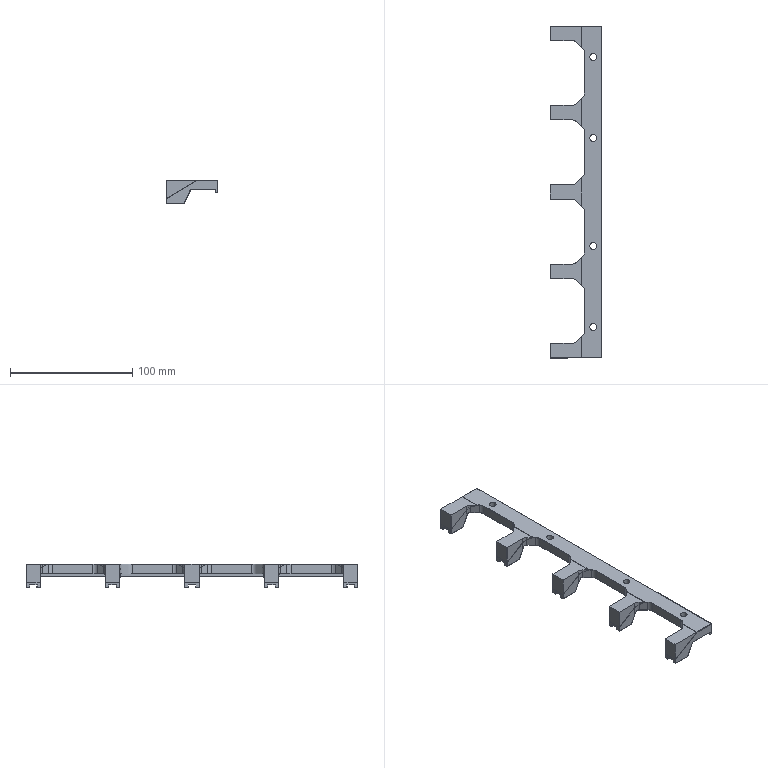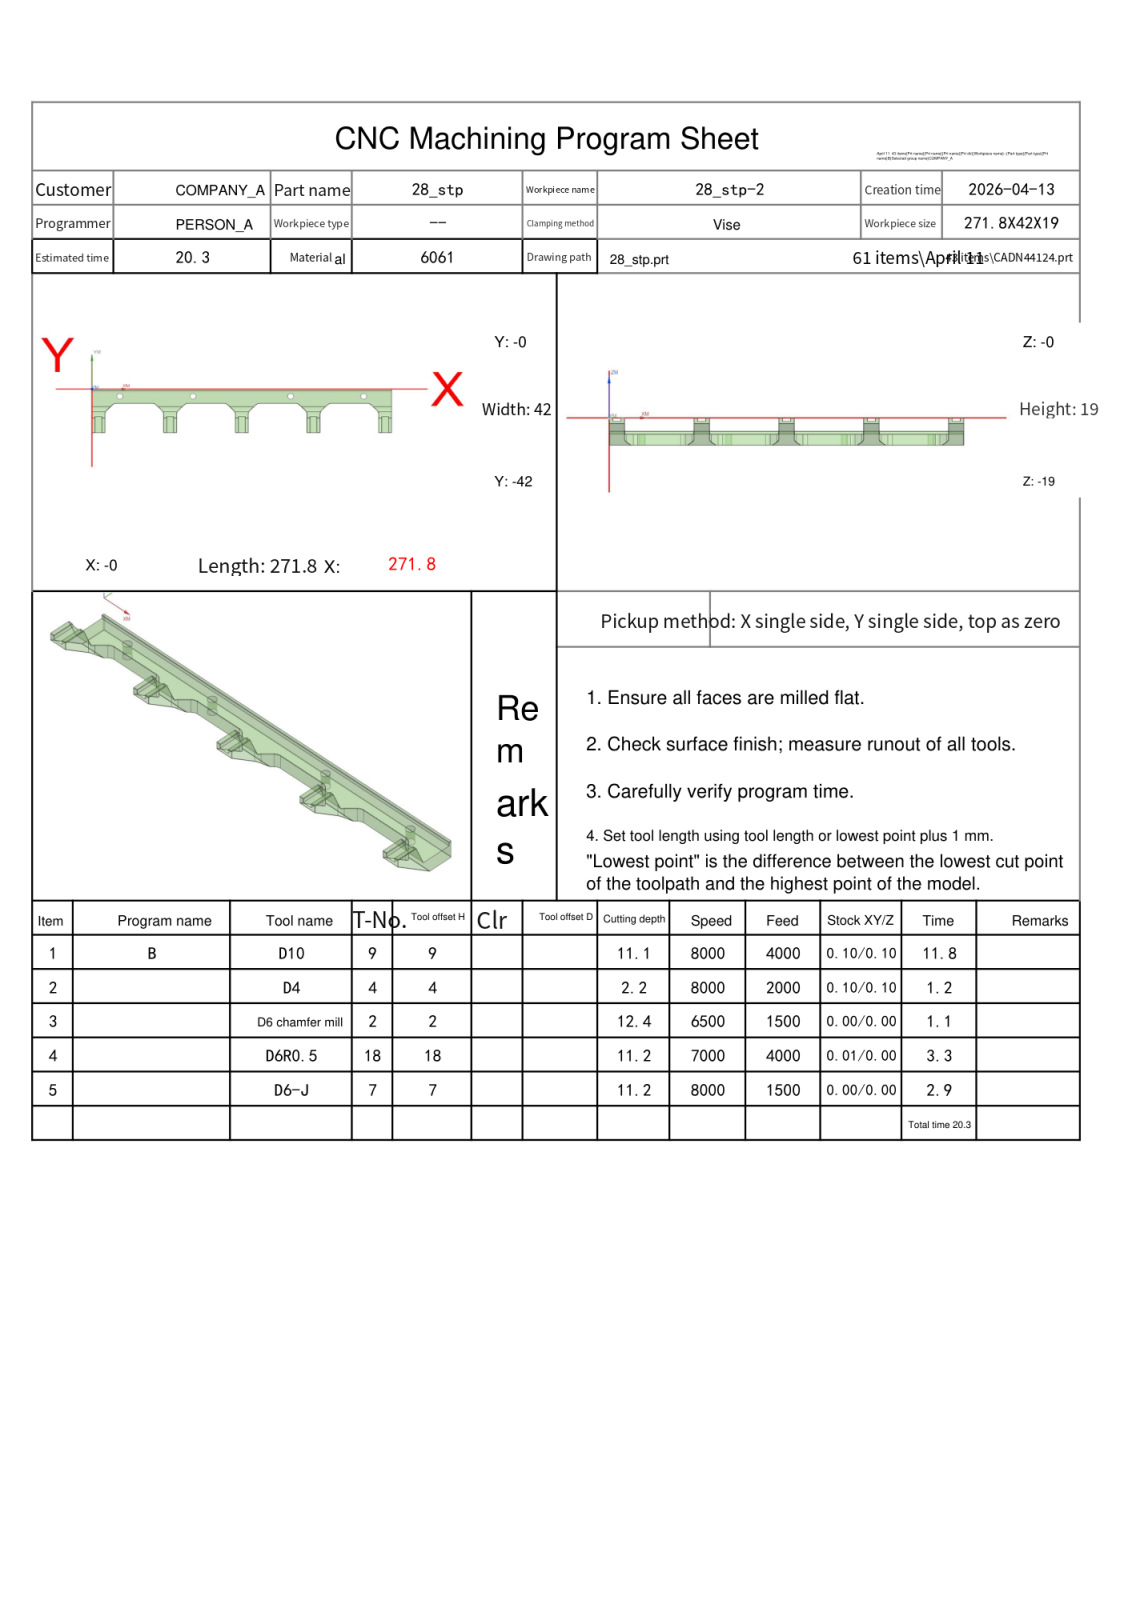NC program | NX | posted by the shop | part box 42 x 271.8 x 19 mm
Lines 7628 to 8696 of 14465:
N4 T18 M06
(D6R0.5  D=6. R=0.5 H=18 ce=0.01 di=0.00)
G00 G90 G54 X253.27 Y-27.629 M03 S7000
G43 H18 Z15.8
M08
Z.447
G01 Z-.053 F4000.
G03 X254.609 Y-27.944 I1.338 J2.685
X256.92 Y-26.857 I0.0 J3.
G02 X257.736 Y-25.975 I8.281 J-6.85
X259.802 Y-25.09 I2.255 J-2.408
G01 X262.9 Y-25.088
G02 X264.966 Y-25.891 I-.055 J-3.199
X265.858 Y-26.823 I-6.91 J-7.504
G01 X265.898 Y-26.869
X265.915 Y-26.85
G02 X266.687 Y-26.023 I12.598 J-10.979
X268.753 Y-25.092 I2.328 J-2.409
G01 X268.925 Y-25.088
X271.734
G02 X273.985 Y-25.998 I0.0 J-3.24
X274.759 Y-26.825 I-7.84 J-8.116
G01 Y-26.799 Z-.105
G03 X273.917 Y-25.896 I-10.451 J-8.901
X271.748 Y-25.003 I-2.234 J-2.346
G01 X268.952
G03 X266.725 Y-25.95 I.099 J-3.323
X265.898 Y-26.843 I15.388 J-15.091
G01 X265.858 Y-26.797
G03 X264.966 Y-25.852 I-9.175 J-7.76
X262.848 Y-25.003 I-2.177 J-2.366
G01 X259.952
G03 X257.736 Y-25.938 I.084 J-3.291
X256.92 Y-26.831 I8.923 J-8.978
G01 Y-26.805 Z-.158
G02 X257.736 Y-25.906 I11.122 J-9.282
X260.004 Y-24.918 I2.338 J-2.269
G01 X262.796
G02 X264.966 Y-25.812 I-.092 J-3.303
G01 X265.111 Y-25.95
X265.736 Y-26.634
X265.859 Y-26.772
X265.898 Y-26.816
X266.686 Y-25.95
G02 X269.004 Y-24.918 I2.434 J-2.345
G01 X271.696
G02 X273.917 Y-25.859 I-.094 J-3.315
G01 X274.012 Y-25.95
X274.762 Y-26.776
Y-26.75 Z-.21
X274.04 Y-25.95
X273.917 Y-25.822
G03 X271.643 Y-24.833 I-2.386 J-2.377
G01 X269.057
G03 X266.661 Y-25.95 I.089 J-3.316
G01 X265.898 Y-26.79
X265.859 Y-26.746
X265.144 Y-25.95
X264.966 Y-25.773
G03 X262.743 Y-24.833 I-2.303 J-2.346
G01 X260.057
G03 X258.021 Y-25.608 I.064 J-3.227
G01 X257.736 Y-25.874
X257.657 Y-25.95
X257.041 Y-26.634
X256.92 Y-26.779
X256.919 Y-26.752 Z-.264
G02 X257.974 Y-25.608 I12.038 J-10.043
X260.112 Y-24.747 I2.203 J-2.384
G01 X262.691
G02 X264.966 Y-25.738 I-.091 J-3.317
X265.86 Y-26.72 I-21.948 J-20.865
G01 X265.898 Y-26.763
X266.636 Y-25.95
X266.687 Y-25.887
X266.974 Y-25.608
G02 X269.104 Y-24.747 I2.207 J-2.395
G01 X271.594
G02 X273.917 Y-25.791 I-.094 J-3.315
G01 X274.068 Y-25.95
X274.763 Y-26.724
Y-26.692 Z-.328
X273.917 Y-25.753
X273.774 Y-25.608
G03 X271.598 Y-24.669 I-2.244 J-2.208
G01 X269.106
G03 X266.952 Y-25.585 I.064 J-3.141
X265.898 Y-26.731 I18.412 J-17.995
G01 X265.86 Y-26.688
X265.078 Y-25.822
G03 X264.276 Y-25.138 I-2.992 J-2.699
X262.697 Y-24.669 I-1.588 J-2.453
G01 X260.1
G03 X257.926 Y-25.608 I.079 J-3.17
G01 X257.736 Y-25.803
X256.988 Y-26.634
X256.918 Y-26.719
X256.917 Y-26.679 Z-.407
X256.953 Y-26.634
X257.676 Y-25.827
X257.762 Y-25.73
G02 X258.405 Y-25.15 I2.847 J-2.508
X260.104 Y-24.606 I1.699 J-2.381
G01 X262.689
X262.699
G02 X264.469 Y-25.203 I0.0 J-2.924
X264.957 Y-25.648 I-2.232 J-2.934
G01 X265.31 Y-26.034
X265.861 Y-26.65
X265.898 Y-26.692
X265.953 Y-26.634
X266.676 Y-25.827
X266.762 Y-25.73
G02 X267.261 Y-25.257 I3.183 J-2.858
X269.107 Y-24.606 I1.852 J-2.308
G01 X271.592
G02 X273.824 Y-25.608 I-.022 J-3.035
G01 X273.917 Y-25.708
X274.764 Y-26.654
X274.696 Y-26.533 Z-.495
X274.024 Y-25.782
X273.85 Y-25.587
G03 X271.6 Y-24.558 I-2.275 J-2.001
G01 X269.093
G03 X266.982 Y-25.452 I0.0 J-2.941
G01 X266.85 Y-25.587
X266.676 Y-25.782
X265.956 Y-26.587
X265.898 Y-26.648
X265.77 Y-26.505
X264.977 Y-25.618
X264.95 Y-25.587
G03 X262.7 Y-24.558 I-2.275 J-2.001
G01 X260.1
G03 X257.85 Y-25.587 I.026 J-3.03
G01 X257.676 Y-25.782
X256.914 Y-26.634
X256.916 Y-26.591 Z-.585
X257.048 Y-26.44
X257.676 Y-25.738
X257.868 Y-25.523
G02 X260.1 Y-24.514 I2.244 J-1.991
G01 X262.7
G02 X264.932 Y-25.523 I-.012 J-3.
G01 X265.016 Y-25.617
X265.776 Y-26.467
X265.898 Y-26.603
X265.999 Y-26.494
X266.676 Y-25.738
X266.876 Y-25.514
G02 X267.029 Y-25.359 I4.931 J-4.721
X269.099 Y-24.514 I2.07 J-2.112
G01 X271.6
G02 X273.832 Y-25.523 I-.012 J-3.
G01 X274.024 Y-25.738
X274.605 Y-26.387
X274.714 Y-26.511
X274.725 Y-26.498 Z-.629
X274.733 Y-26.488 Z-.674
X274.605 Y-26.342
X274.024 Y-25.693
X273.826 Y-25.471
G03 X271.6 Y-24.469 I-2.234 J-1.988
G01 X269.097
G03 X267.121 Y-25.228 I0.0 J-2.95
X266.876 Y-25.469 I2.648 J-2.937
G01 X266.676 Y-25.693
X265.999 Y-26.45
X265.898 Y-26.558
X265.779 Y-26.425
X265.049 Y-25.608
X264.926 Y-25.472
G03 X262.7 Y-24.469 I-2.234 J-1.988
G01 X260.1
G03 X257.874 Y-25.472 I.008 J-2.99
G01 X257.676 Y-25.693
X257.048 Y-26.395
X256.917 Y-26.548
Y-26.504 Z-.763
X257.048 Y-26.35
X257.676 Y-25.648
X257.876 Y-25.425
G02 X260.1 Y-24.424 I2.231 J-1.987
G01 X262.7
G02 X264.924 Y-25.425 I-.006 J-2.987
G01 X265.089 Y-25.608
X265.799 Y-26.403
X265.898 Y-26.513
X265.999 Y-26.405
X266.676 Y-25.648
X266.876 Y-25.425
G02 X269.1 Y-24.424 I2.252 J-2.035
G01 X271.6
G02 X273.824 Y-25.425 I-.006 J-2.987
G01 X274.024 Y-25.648
X274.751 Y-26.466
X274.786 Y-26.463 Z-.853
X274.641 Y-26.292
X274.024 Y-25.604
X273.824 Y-25.38
G03 X271.6 Y-24.38 I-2.231 J-1.987
G01 X269.1
G03 X266.876 Y-25.38 I.006 J-2.987
G01 X266.676 Y-25.604
X265.999 Y-26.36
X265.898 Y-26.469
X265.819 Y-26.38
X265.124 Y-25.604
X264.924 Y-25.38
G03 X262.7 Y-24.38 I-2.231 J-1.987
G01 X260.1
G03 X257.876 Y-25.38 I.006 J-2.987
G01 X257.676 Y-25.604
X257.048 Y-26.306
X256.917 Y-26.46
Y-26.416 Z-.942
X257.02 Y-26.292
X257.676 Y-25.559
X257.876 Y-25.335
G02 X260.1 Y-24.335 I2.231 J-1.987
G01 X262.7
G02 X264.924 Y-25.335 I-.006 J-2.987
G01 X265.124 Y-25.559
X265.839 Y-26.358
X265.898 Y-26.424
X265.999 Y-26.316
X266.676 Y-25.559
X266.876 Y-25.335
G02 X269.1 Y-24.335 I2.231 J-1.987
G01 X271.6
G02 X273.824 Y-25.335 I-.006 J-2.987
G01 X274.024 Y-25.559
X274.681 Y-26.292
X274.815 Y-26.453
X274.829 Y-26.438 Z-.987
X274.835 Y-26.43 Z-1.032
X274.721 Y-26.292
X274.024 Y-25.514
X273.824 Y-25.29
G03 X271.6 Y-24.29 I-2.231 J-1.987
G01 X269.1
G03 X266.876 Y-25.29 I.006 J-2.987
G01 X266.676 Y-25.514
X265.98 Y-26.292
X265.898 Y-26.379
X265.859 Y-26.336
X265.124 Y-25.514
X264.924 Y-25.29
G03 X262.7 Y-24.29 I-2.231 J-1.987
G01 X260.1
G03 X257.876 Y-25.29 I.006 J-2.987
G01 X257.676 Y-25.514
X256.98 Y-26.292
X256.915 Y-26.371
X256.913 Y-26.325 Z-1.121
X256.939 Y-26.292
X257.676 Y-25.469
X257.876 Y-25.246
G02 X260.1 Y-24.245 I2.231 J-1.987
G01 X262.7
G02 X264.924 Y-25.246 I-.006 J-2.987
G01 X265.124 Y-25.469
X265.88 Y-26.313
X265.884 Y-26.34
X265.914
X265.919 Y-26.313
X265.939 Y-26.292
X266.676 Y-25.469
X266.876 Y-25.246
G02 X269.1 Y-24.245 I2.231 J-1.987
G01 X271.6
G02 X273.824 Y-25.246 I-.006 J-2.987
G01 X274.024 Y-25.469
X274.761 Y-26.292
X274.855 Y-26.408
X274.77 Y-26.26 Z-1.211
X274.024 Y-25.425
X273.824 Y-25.201
G03 X271.6 Y-24.201 I-2.231 J-1.987
G01 X269.1
G03 X266.865 Y-25.213 I.014 J-3.005
G01 X266.676 Y-25.425
X265.94 Y-26.247
X265.9 Y-26.292
X265.779 Y-26.157
X265.124 Y-25.425
X264.924 Y-25.201
G03 X262.7 Y-24.201 I-2.231 J-1.987
G01 X260.1
G03 X257.876 Y-25.201 I.006 J-2.987
G01 X257.676 Y-25.425
X256.912 Y-26.28
X256.913 Y-26.237 Z-1.3
X257.048 Y-26.082
X257.676 Y-25.38
X257.876 Y-25.156
G02 X260.1 Y-24.156 I2.231 J-1.987
G01 X262.7
G02 X264.924 Y-25.156 I-.006 J-2.987
G01 X265.124 Y-25.38
X265.673 Y-25.993
X265.9 Y-26.247
X265.99 Y-26.147
X266.676 Y-25.38
X266.818 Y-25.22
X266.792 Y-25.191
X266.822 Y-25.158
X266.854 Y-25.181
X266.876 Y-25.156
G02 X269.1 Y-24.156 I2.231 J-1.987
G01 X271.6
G02 X273.824 Y-25.156 I-.006 J-2.987
G01 X274.024 Y-25.38
X274.769 Y-26.217
Y-26.174 Z-1.39
X274.024 Y-25.335
X273.824 Y-25.112
G03 X271.6 Y-24.111 I-2.231 J-1.987
G01 X269.1
G03 X268.395 Y-24.194 I.011 J-3.136
G01 X268.534 Y-24.157 Z-1.407
X268.674 Y-24.124 Z-1.425
X268.816 Y-24.098 Z-1.443
X268.958 Y-24.079 Z-1.461
X269.1 Y-24.066 Z-1.479
X271.6
G02 X273.824 Y-25.067 I-.012 J-3.
G01 X274.024 Y-25.291
X274.769 Y-26.131
X274.77 Y-26.087 Z-1.568
X274.655 Y-25.95
X274.024 Y-25.246
X273.824 Y-25.022
G03 X271.6 Y-24.022 I-2.233 J-1.992
G01 X269.1
G00 Z15.8
X253.277 Y-26.914
Z-.89
G01 Z-1.39
G03 X254.637 Y-27.24 I1.359 J2.674
X256.914 Y-26.193 I0.0 J3.
G01 X257.048 Y-26.037
X257.676 Y-25.335
X257.876 Y-25.112
G02 X260.1 Y-24.111 I2.231 J-1.987
G01 X262.7
G02 X263.406 Y-24.194 I-.092 J-3.829
G01 X263.267 Y-24.157 Z-1.407
X263.126 Y-24.124 Z-1.425
X262.984 Y-24.098 Z-1.443
X262.842 Y-24.079 Z-1.461
X262.7 Y-24.066 Z-1.479
X260.1
G03 X257.876 Y-25.067 I.006 J-2.987
G01 X257.676 Y-25.291
X257.048 Y-25.992
X256.914 Y-26.15
Y-26.106 Z-1.568
X257.045 Y-25.95
X257.676 Y-25.246
X257.876 Y-25.022
G02 X260.1 Y-24.022 I2.231 J-1.987
G01 X262.7
G00 Z15.8
X278.416 Y-26.795
Z-1.158
G01 Z-1.658
G02 X277.07 Y-27.114 I-1.346 J2.681
X274.772 Y-26.042 I0.0 J3.
G01 X274.695 Y-25.95
X274.024 Y-25.201
X273.824 Y-24.977
G03 X271.6 Y-23.977 I-2.231 J-1.987
G01 X260.1
G03 X257.876 Y-24.977 I.006 J-2.987
G01 X257.676 Y-25.201
X257.005 Y-25.95
X256.913 Y-26.061
X256.912 Y-26.016 Z-1.747
X256.965 Y-25.95
X257.676 Y-25.156
X257.876 Y-24.933
G02 X260.1 Y-23.932 I2.231 J-1.987
G01 X271.6
G02 X273.824 Y-24.933 I-.006 J-2.987
G01 X274.024 Y-25.156
X274.735 Y-25.95
X274.774 Y-25.997
X274.776 Y-25.952 Z-1.837
X274.024 Y-25.112
X273.824 Y-24.888
G03 X271.6 Y-23.888 I-2.231 J-1.987
G01 X260.1
G03 X257.876 Y-24.888 I.006 J-2.987
G01 X257.676 Y-25.112
X256.925 Y-25.95
X256.91 Y-25.97
X256.909 Y-25.926 Z-1.926
X257.048 Y-25.769
X257.676 Y-25.067
X257.876 Y-24.843
G02 X260.1 Y-23.843 I2.231 J-1.987
G01 X271.6
G02 X273.824 Y-24.843 I-.006 J-2.987
G01 X274.024 Y-25.067
X274.775 Y-25.909
Y-25.866 Z-2.016
X274.024 Y-25.022
X273.824 Y-24.799
G03 X271.6 Y-23.798 I-2.231 J-1.987
G01 X260.1
G03 X257.876 Y-24.799 I.006 J-2.987
G01 X257.676 Y-25.022
X257.048 Y-25.724
X256.911 Y-25.882
Y-25.839 Z-2.105
X257.048 Y-25.679
X257.676 Y-24.977
X257.876 Y-24.754
G02 X260.1 Y-23.753 I2.231 J-1.987
G01 X271.6
G02 X273.824 Y-24.754 I-.006 J-2.987
G01 X274.024 Y-24.977
X274.775 Y-25.823
Y-25.779 Z-2.195
X274.629 Y-25.608
X274.024 Y-24.933
X273.824 Y-24.709
G03 X271.6 Y-23.709 I-2.238 J-2.003
G01 X260.1
G03 X257.876 Y-24.709 I.006 J-2.987
G01 X257.676 Y-24.933
X257.048 Y-25.635
X256.912 Y-25.795
Y-25.751 Z-2.284
X257.031 Y-25.608
X257.876 Y-24.664
G02 X260.1 Y-23.664 I2.231 J-1.987
G01 X271.6
G02 X273.824 Y-24.664 I-.006 J-2.987
G01 X274.024 Y-24.888
X274.669 Y-25.608
X274.776 Y-25.735
X274.778 Y-25.69 Z-2.373
X274.709 Y-25.608
X274.024 Y-24.843
X273.824 Y-24.62
G03 X271.6 Y-23.619 I-2.231 J-1.987
G01 X260.1
G03 X257.876 Y-24.62 I.006 J-2.987
G01 X256.991 Y-25.608
X256.911 Y-25.706
X256.909 Y-25.66 Z-2.463
X256.951 Y-25.608
X257.876 Y-24.575
G02 X260.1 Y-23.575 I2.231 J-1.987
G01 X271.6
G02 X273.824 Y-24.575 I-.006 J-2.987
G01 X274.024 Y-24.799
X274.749 Y-25.608
X274.78 Y-25.645
X274.782 Y-25.6 Z-2.552
X274.024 Y-24.754
X273.824 Y-24.53
G03 X271.6 Y-23.53 I-2.231 J-1.987
G01 X260.1
G03 X257.876 Y-24.53 I.006 J-2.987
G01 X257.676 Y-24.754
X256.907 Y-25.614
X256.908 Y-25.571 Z-2.642
X257.048 Y-25.411
X257.876 Y-24.485
G02 X260.1 Y-23.485 I2.231 J-1.987
G01 X271.6
G02 X273.824 Y-24.485 I-.006 J-2.987
G01 X274.024 Y-24.709
X274.781 Y-25.558
X274.78 Y-25.514 Z-2.731
X274.024 Y-24.664
X273.824 Y-24.441
G03 X271.6 Y-23.44 I-2.231 J-1.987
G01 X260.1
G03 X257.876 Y-24.441 I.006 J-2.987
G01 X257.048 Y-25.366
X256.909 Y-25.528
Y-25.484 Z-2.821
X257.048 Y-25.322
X257.876 Y-24.396
G02 X260.1 Y-23.396 I2.231 J-1.987
G01 X271.6
G02 X273.824 Y-24.396 I-.009 J-2.992
G01 X274.024 Y-24.62
X274.78 Y-25.471
X274.781 Y-25.427 Z-2.91
X274.643 Y-25.266
X274.024 Y-24.575
X273.824 Y-24.351
G03 X271.6 Y-23.351 I-2.237 J-2.001
G01 X260.1
G03 X257.876 Y-24.351 I.006 J-2.987
G01 X257.048 Y-25.277
X256.91 Y-25.44
X256.909 Y-25.395 Z-3.
X257.017 Y-25.266
X257.876 Y-24.307
G02 X260.1 Y-23.306 I2.231 J-1.987
G01 X271.6
G02 X273.824 Y-24.307 I-.006 J-2.987
G01 X274.024 Y-24.53
X274.683 Y-25.266
X274.782 Y-25.382
X274.783 Y-25.338 Z-3.089
X274.723 Y-25.266
X274.024 Y-24.486
X273.824 Y-24.262
G03 X271.6 Y-23.261 I-2.231 J-1.987
G01 X260.1
G03 X257.876 Y-24.262 I.006 J-2.987
G01 X256.977 Y-25.266
X256.908 Y-25.35
X256.906 Y-25.304 Z-3.178
X256.937 Y-25.266
X257.876 Y-24.217
G02 X260.1 Y-23.217 I2.231 J-1.987
G01 X271.6
G02 X273.824 Y-24.217 I-.006 J-2.987
G01 X274.024 Y-24.441
X274.763 Y-25.266
X274.785 Y-25.292
X274.786 Y-25.248 Z-3.268
X274.024 Y-24.396
X273.824 Y-24.172
G03 X271.6 Y-23.172 I-2.231 J-1.987
G01 X260.1
G03 X257.876 Y-24.172 I.006 J-2.987
G01 X257.676 Y-24.396
X256.904 Y-25.259
X256.906 Y-25.216 Z-3.357
X257.048 Y-25.053
X257.876 Y-24.128
G02 X260.1 Y-23.127 I2.231 J-1.987
G01 X271.6
G02 X273.824 Y-24.128 I-.006 J-2.987
G01 X274.024 Y-24.351
X274.785 Y-25.205
Y-25.162 Z-3.447
X274.024 Y-24.307
X273.824 Y-24.083
G03 X271.6 Y-23.083 I-2.231 J-1.987
G01 X260.1
G03 X257.876 Y-24.083 I.006 J-2.987
G01 X257.048 Y-25.009
X256.907 Y-25.172
Y-25.129 Z-3.536
X257.048 Y-24.964
X257.876 Y-24.038
G02 X260.1 Y-23.038 I2.231 J-1.987
G01 X271.6
G02 X273.824 Y-24.038 I-.012 J-3.001
G01 X274.024 Y-24.262
X274.785 Y-25.118
Y-25.074 Z-3.626
X274.657 Y-24.924
X274.024 Y-24.217
X273.824 Y-23.994
G03 X271.6 Y-22.993 I-2.232 J-1.989
G01 X260.1
G03 X257.876 Y-23.994 I.006 J-2.987
G01 X257.043 Y-24.924
X256.908 Y-25.085
X256.907 Y-25.04 Z-3.715
X257.003 Y-24.924
X257.876 Y-23.949
G02 X260.1 Y-22.948 I2.231 J-1.987
G01 X271.6
G02 X273.824 Y-23.949 I-.006 J-2.987
G01 X274.024 Y-24.172
X274.697 Y-24.924
X274.787 Y-25.03
X274.788 Y-24.985 Z-3.805
X274.738 Y-24.924
X274.024 Y-24.128
X273.824 Y-23.904
G03 X271.6 Y-22.904 I-2.231 J-1.987
G01 X260.1
G03 X257.876 Y-23.904 I.006 J-2.987
G01 X256.963 Y-24.924
X256.905 Y-24.994
X256.903 Y-24.949 Z-3.894
X256.923 Y-24.924
X257.876 Y-23.859
G02 X260.1 Y-22.859 I2.231 J-1.987
G01 X271.6
G02 X273.824 Y-23.859 I-.006 J-2.987
G01 X274.024 Y-24.083
X274.79 Y-24.94
Y-24.896 Z-3.983
X274.024 Y-24.038
X273.824 Y-23.815
G03 X271.6 Y-22.814 I-2.231 J-1.987
G01 X260.1
G03 X257.876 Y-23.815 I.006 J-2.987
G01 X257.048 Y-24.74
X256.903 Y-24.904
X256.904 Y-24.861 Z-4.073
X257.048 Y-24.695
X257.876 Y-23.77
G02 X260.1 Y-22.77 I2.231 J-1.987
G01 X271.6
G02 X273.824 Y-23.77 I-.006 J-2.987
G01 X274.024 Y-23.994
X274.789 Y-24.852
Y-24.809 Z-4.162
X274.024 Y-23.949
X273.824 Y-23.725
G03 X271.6 Y-22.725 I-2.231 J-1.987
G01 X260.1
G03 X257.876 Y-23.725 I.006 J-2.987
G01 X257.048 Y-24.651
X256.905 Y-24.817
X256.906 Y-24.773 Z-4.252
X257.048 Y-24.606
X257.876 Y-23.681
G02 X260.1 Y-22.68 I2.231 J-1.987
G01 X271.6
G02 X273.824 Y-23.681 I-.014 J-3.004
G01 X274.024 Y-23.904
X274.789 Y-24.765
Y-24.72 Z-4.341
X274.672 Y-24.582
X274.024 Y-23.859
X273.824 Y-23.636
G03 X271.6 Y-22.635 I-2.231 J-1.987
G01 X260.1
G03 X257.876 Y-23.636 I.006 J-2.987
G01 X257.029 Y-24.582
X256.906 Y-24.728
X256.905 Y-24.683 Z-4.431
X256.989 Y-24.582
X257.876 Y-23.591
G02 X260.1 Y-22.591 I2.231 J-1.987
G01 X271.6
G02 X273.824 Y-23.591 I-.006 J-2.987
G01 X274.024 Y-23.815
X274.712 Y-24.582
X274.79 Y-24.675
X274.792 Y-24.63 Z-4.52
X274.752 Y-24.582
X274.024 Y-23.77
X273.824 Y-23.546
G03 X271.6 Y-22.546 I-2.231 J-1.987
G01 X260.1
G03 X257.876 Y-23.546 I.006 J-2.987
G01 X256.949 Y-24.582
X256.904 Y-24.637
X256.902 Y-24.591 Z-4.609
X257.676 Y-23.725
X257.876 Y-23.502
G02 X260.1 Y-22.501 I2.231 J-1.987
G01 X271.6
G02 X273.824 Y-23.502 I-.006 J-2.987
G01 X274.024 Y-23.725
X274.793 Y-24.584
X274.792 Y-24.541 Z-4.699
X274.024 Y-23.681
X273.824 Y-23.457
G03 X271.6 Y-22.457 I-2.231 J-1.987
G01 X260.1
G03 X257.876 Y-23.457 I.006 J-2.987
G01 X257.048 Y-24.382
X256.903 Y-24.548
X256.904 Y-24.504 Z-4.788
X257.048 Y-24.338
X257.876 Y-23.412
G02 X260.1 Y-22.412 I2.231 J-1.987
G01 X271.6
G02 X273.824 Y-23.412 I-.006 J-2.987
G01 X274.024 Y-23.636
X274.792 Y-24.498
X274.791 Y-24.454 Z-4.878
X274.024 Y-23.591
X273.824 Y-23.367
G03 X271.6 Y-22.367 I-2.234 J-1.994
G01 X260.1
G03 X257.876 Y-23.367 I.006 J-2.987
G01 X257.048 Y-24.293
X256.905 Y-24.46
Y-24.416 Z-4.967
X257.048 Y-24.248
X257.876 Y-23.323
G02 X260.1 Y-22.322 I2.231 J-1.987
G01 X271.6
G02 X273.824 Y-23.323 I-.012 J-3.
G01 X274.024 Y-23.546
X274.646 Y-24.24
X274.791 Y-24.41
X274.792 Y-24.365 Z-5.057
X274.686 Y-24.24
X274.024 Y-23.502
X273.824 Y-23.278
G03 X271.6 Y-22.278 I-2.231 J-1.987
G01 X260.1
G03 X257.876 Y-23.278 I.006 J-2.987
G01 X257.015 Y-24.24
X256.905 Y-24.371
X256.904 Y-24.326 Z-5.146
X256.975 Y-24.24
X257.876 Y-23.233
G02 X260.1 Y-22.233 I2.231 J-1.987
G01 X271.6
G02 X273.824 Y-23.233 I-.006 J-2.987
G01 X274.024 Y-23.457
X274.726 Y-24.24
X274.793 Y-24.32
X274.795 Y-24.275 Z-5.236
X274.766 Y-24.24
X274.024 Y-23.412
X273.824 Y-23.189
G03 X271.6 Y-22.188 I-2.231 J-1.987
G01 X260.1
G03 X257.876 Y-23.189 I.006 J-2.987
G01 X256.935 Y-24.24
X256.902 Y-24.28
X256.901 Y-24.234 Z-5.325
X257.676 Y-23.367
X257.876 Y-23.144
G02 X260.1 Y-22.143 I2.231 J-1.987
G01 X271.6
G02 X273.824 Y-23.144 I-.006 J-2.987
G01 X274.024 Y-23.367
X274.796 Y-24.23
X274.794 Y-24.186 Z-5.414
X274.024 Y-23.323
X273.824 Y-23.099
G03 X271.6 Y-22.099 I-2.231 J-1.987
G01 X260.1
G03 X257.876 Y-23.099 I.006 J-2.987
G01 X257.048 Y-24.025
X256.902 Y-24.191
X256.903 Y-24.147 Z-5.504
X257.048 Y-23.98
X257.876 Y-23.054
G02 X260.1 Y-22.054 I2.231 J-1.987
G01 X271.6
G02 X273.824 Y-23.054 I-.006 J-2.987
G01 X274.024 Y-23.278
X274.794 Y-24.143
X274.793 Y-24.099 Z-5.593
X274.024 Y-23.233
X273.824 Y-23.01
G03 X271.6 Y-22.009 I-2.237 J-2.001
G01 X260.1
G03 X257.876 Y-23.01 I.006 J-2.987
G01 X257.048 Y-23.935
X256.904 Y-24.103
X256.905 Y-24.059 Z-5.683
X257.041 Y-23.898
X257.876 Y-22.965
G02 X260.1 Y-21.965 I2.231 J-1.987
G01 X271.6
G02 X273.824 Y-22.965 I-.006 J-2.987
G01 X274.024 Y-23.189
X274.66 Y-23.898
X274.793 Y-24.054
X274.794 Y-24.009 Z-5.772
X274.7 Y-23.898
X274.024 Y-23.144
X273.824 Y-22.92
G03 X271.6 Y-21.92 I-2.231 J-1.987
G01 X260.1
G03 X257.876 Y-22.92 I.006 J-2.987
G01 X257.001 Y-23.898
X256.904 Y-24.014
X256.903 Y-23.968 Z-5.862
X256.961 Y-23.898
X257.876 Y-22.876
G02 X260.1 Y-21.875 I2.231 J-1.987
G01 X271.6
G02 X273.824 Y-22.876 I-.006 J-2.987
G01 X274.024 Y-23.099
X274.74 Y-23.898
X274.795 Y-23.964
X274.796 Y-23.918 Z-5.951
X274.024 Y-23.054
X273.824 Y-22.831
G03 X271.6 Y-21.83 I-2.231 J-1.987
G01 X260.1
G03 X257.876 Y-22.831 I.006 J-2.987
G01 X256.921 Y-23.898
X256.901 Y-23.922
Y-23.877 Z-6.041
X257.048 Y-23.712
X257.876 Y-22.786
G02 X260.1 Y-21.786 I2.231 J-1.987
G01 X271.6
G02 X273.824 Y-22.786 I-.006 J-2.987
G01 X274.024 Y-23.01
X274.796 Y-23.874
X274.795 Y-23.83 Z-6.13
X274.024 Y-22.965
X273.824 Y-22.741
G03 X271.6 Y-21.741 I-2.231 J-1.987
G01 X260.1
G03 X257.876 Y-22.741 I.006 J-2.987
G01 X257.048 Y-23.667
X256.903 Y-23.834
X256.904 Y-23.79 Z-6.219
X257.048 Y-23.622
X257.876 Y-22.697
G02 X260.1 Y-21.696 I2.231 J-1.987
G01 X271.6
G02 X273.824 Y-22.697 I-.006 J-2.987
G01 X274.024 Y-22.92
X274.795 Y-23.786
X274.794 Y-23.742 Z-6.309
X274.024 Y-22.876
X273.824 Y-22.652
G03 X271.6 Y-21.652 I-2.238 J-2.003
G01 X260.1
G03 X257.876 Y-22.652 I.006 J-2.987
G01 X257.048 Y-23.577
X256.904 Y-23.746
X256.905 Y-23.701 Z-6.398
X257.027 Y-23.556
X257.876 Y-22.607
G02 X260.1 Y-21.607 I2.231 J-1.987
G01 X271.6
G02 X273.824 Y-22.607 I-.006 J-2.987
G01 X274.024 Y-22.831
X274.674 Y-23.556
X274.795 Y-23.697
Y-23.652 Z-6.488
X274.714 Y-23.556
X274.024 Y-22.786
X273.824 Y-22.562
G03 X271.6 Y-21.562 I-2.231 J-1.987
G01 X260.1
G03 X257.876 Y-22.562 I.006 J-2.987
G01 X256.987 Y-23.556
X256.904 Y-23.656
X256.903 Y-23.61 Z-6.577
X256.947 Y-23.556
X257.876 Y-22.518
G02 X260.1 Y-21.517 I2.231 J-1.987
G01 X271.6
G02 X273.824 Y-22.518 I-.006 J-2.987
G01 X274.024 Y-22.741
X274.754 Y-23.556
X274.796 Y-23.607
X274.798 Y-23.561 Z-6.667
X274.024 Y-22.697
X273.824 Y-22.473
G03 X271.6 Y-21.473 I-2.231 J-1.987
G01 X260.1
G03 X257.876 Y-22.473 I.006 J-2.987
G01 X257.676 Y-22.697
X256.901 Y-23.564
X256.902 Y-23.52 Z-6.756
X257.048 Y-23.354
X257.876 Y-22.428
G02 X260.1 Y-21.428 I2.231 J-1.987
G01 X271.6
G02 X273.824 Y-22.428 I-.006 J-2.987
G01 X274.024 Y-22.652
X274.797 Y-23.517
X274.796 Y-23.473 Z-6.846
X274.024 Y-22.607
X273.824 Y-22.384
G03 X271.6 Y-21.383 I-2.231 J-1.987
G01 X260.1
G03 X257.876 Y-22.384 I.006 J-2.987
G01 X257.048 Y-23.309
X256.903 Y-23.476
X256.904 Y-23.432 Z-6.935
X257.048 Y-23.264
X257.876 Y-22.339
G02 X260.1 Y-21.338 I2.231 J-1.987
G01 X271.6
G02 X273.824 Y-22.339 I-.01 J-2.995
G01 X274.024 Y-22.563
X274.795 Y-23.429
Y-23.385 Z-7.024
X274.648 Y-23.214
X274.024 Y-22.518
X273.824 Y-22.294
G03 X271.6 Y-21.294 I-2.236 J-1.998
G01 X260.1
G03 X257.876 Y-22.294 I.006 J-2.987
G01 X257.048 Y-23.22
X256.905 Y-23.388
Y-23.343 Z-7.114
X257.013 Y-23.214
X257.876 Y-22.249
G02 X260.1 Y-21.249 I2.231 J-1.987
G01 X271.6
G02 X273.824 Y-22.249 I-.006 J-2.987
G01 X274.024 Y-22.473
X274.688 Y-23.214
X274.795 Y-23.34
X274.796 Y-23.294 Z-7.203
X274.728 Y-23.214
X274.024 Y-22.428
X273.824 Y-22.205
G03 X271.6 Y-21.204 I-2.231 J-1.987
G01 X260.1
G03 X257.876 Y-22.205 I.006 J-2.987
G01 X256.973 Y-23.214
X256.904 Y-23.297
X256.903 Y-23.251 Z-7.293
X256.933 Y-23.214
X257.876 Y-22.16
G02 X260.1 Y-21.16 I2.231 J-1.987
G01 X271.6
G02 X273.824 Y-22.16 I-.006 J-2.987
G01 X274.024 Y-22.384
X274.768 Y-23.214
X274.797 Y-23.249
X274.798 Y-23.203 Z-7.382
X274.024 Y-22.339
X273.824 Y-22.115
G03 X271.6 Y-21.115 I-2.231 J-1.987
G01 X260.1
G03 X257.876 Y-22.115 I.006 J-2.987
G01 X257.676 Y-22.339
X256.901 Y-23.205
X256.903 Y-23.162 Z-7.472
X257.048 Y-22.996
X257.876 Y-22.071
G02 X260.1 Y-21.07 I2.231 J-1.987
G01 X271.6
G02 X273.824 Y-22.071 I-.006 J-2.987
G01 X274.024 Y-22.294
X274.796 Y-23.16
X274.795 Y-23.116 Z-7.561
X274.024 Y-22.249
X273.824 Y-22.026
G03 X271.6 Y-21.025 I-2.231 J-1.987
G01 X260.1
G03 X257.876 Y-22.026 I.006 J-2.987
G01 X257.048 Y-22.951
X256.904 Y-23.118
X256.905 Y-23.074 Z-7.651
X257.048 Y-22.907
X257.876 Y-21.981
G02 X260.1 Y-20.981 I2.231 J-1.987
G01 X271.6
G02 X273.824 Y-21.981 I-.013 J-3.002
G01 X274.024 Y-22.205
X274.794 Y-23.071
Y-23.026 Z-7.74
X274.662 Y-22.872
X274.024 Y-22.16
X273.824 Y-21.936
G03 X271.6 Y-20.936 I-2.231 J-1.987
G01 X260.1
G03 X257.876 Y-21.936 I.006 J-2.987
G01 X257.039 Y-22.872
X256.906 Y-23.029
Y-22.984 Z-7.829
X256.999 Y-22.872
X257.876 Y-21.892
G02 X260.1 Y-20.891 I2.231 J-1.987
G01 X271.6
G02 X273.824 Y-21.892 I-.006 J-2.987
G01 X274.024 Y-22.115
X274.702 Y-22.872
X274.795 Y-22.981
Y-22.935 Z-7.919
X274.742 Y-22.872
X274.024 Y-22.071
X273.824 Y-21.847
G03 X271.6 Y-20.847 I-2.231 J-1.987
G01 X260.1
G03 X257.876 Y-21.847 I.006 J-2.987
G01 X256.959 Y-22.872
X256.905 Y-22.938
X256.903 Y-22.891 Z-8.008
X256.919 Y-22.872
X257.876 Y-21.802
G02 X260.1 Y-20.802 I2.231 J-1.987
G01 X271.6
G02 X273.824 Y-21.802 I-.006 J-2.987
G01 X274.024 Y-22.026
X274.797 Y-22.89
X274.796 Y-22.845 Z-8.098
X274.024 Y-21.981
X273.824 Y-21.757
G03 X271.6 Y-20.757 I-2.231 J-1.987
G01 X260.1
G03 X257.876 Y-21.757 I.006 J-2.987
G01 X257.048 Y-22.683
X256.903 Y-22.847
X256.905 Y-22.803 Z-8.187
X257.048 Y-22.638
X257.876 Y-21.713
G02 X260.1 Y-20.712 I2.231 J-1.987
G01 X271.6
G02 X273.824 Y-21.713 I-.006 J-2.987
G01 X274.024 Y-21.936
X274.795 Y-22.801
X274.794 Y-22.757 Z-8.277
X274.024 Y-21.892
X273.824 Y-21.668
G03 X271.6 Y-20.668 I-2.231 J-1.987
G01 X260.1
G03 X257.876 Y-21.668 I.006 J-2.987
G01 X257.048 Y-22.594
X256.906 Y-22.759
X256.907 Y-22.715 Z-8.366
X257.048 Y-22.549
X257.876 Y-21.623
G02 X260.1 Y-20.623 I2.231 J-1.987
G01 X271.6
G02 X273.824 Y-21.623 I-.014 J-3.003
G01 X274.024 Y-21.847
X274.793 Y-22.713
X274.794 Y-22.668 Z-8.455
X274.676 Y-22.53
X274.024 Y-21.802
X273.824 Y-21.579
G03 X271.6 Y-20.578 I-2.231 J-1.987
G01 X260.1
G03 X257.876 Y-21.579 I.006 J-2.987
G01 X257.025 Y-22.53
X256.907 Y-22.67
Y-22.624 Z-8.545
X256.985 Y-22.53
X257.876 Y-21.534
G02 X260.1 Y-20.534 I2.231 J-1.987
G01 X271.6
G02 X273.824 Y-21.534 I-.006 J-2.987
G01 X274.024 Y-21.758
X274.716 Y-22.53
X274.794 Y-22.622
X274.795 Y-22.577 Z-8.634
X274.756 Y-22.53
X274.024 Y-21.713
X273.824 Y-21.489
G03 X271.6 Y-20.489 I-2.231 J-1.987
G01 X260.1
G03 X257.876 Y-21.489 I.006 J-2.987
G01 X256.945 Y-22.53
X256.905 Y-22.578
X256.904 Y-22.531 Z-8.724
X257.676 Y-21.668
X257.876 Y-21.445
G02 X260.1 Y-20.444 I2.231 J-1.987
G01 X271.6
G02 X273.824 Y-21.445 I-.006 J-2.987
G01 X274.024 Y-21.668
X274.796 Y-22.531
X274.795 Y-22.487 Z-8.813
X274.024 Y-21.624
X273.824 Y-21.4
G03 X271.6 Y-20.399 I-2.231 J-1.987
G01 X260.1
G03 X257.876 Y-21.4 I.006 J-2.987
G01 X257.048 Y-22.325
X256.906 Y-22.488
X256.907 Y-22.444 Z-8.902
X257.048 Y-22.281
X257.876 Y-21.355
G02 X260.1 Y-20.355 I2.231 J-1.987
G01 X271.6
G02 X273.824 Y-21.355 I-.006 J-2.987
G01 X274.024 Y-21.579
X274.793 Y-22.443
X274.792 Y-22.398 Z-8.992
X274.024 Y-21.534